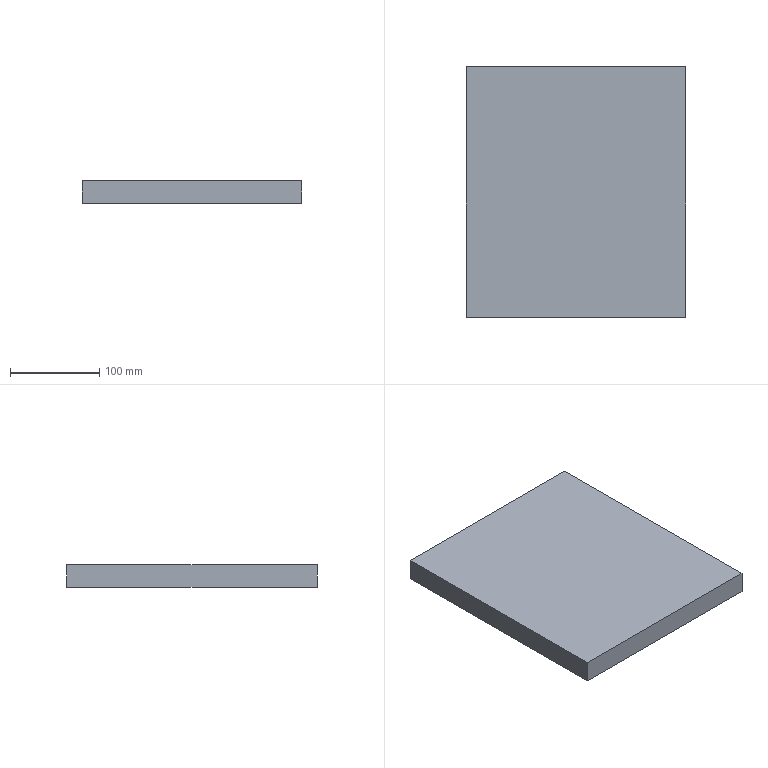Part | SolidWorks | features Extrusion 1 | 1 solid | 6 faces | box 245 x 280 x 25 mm | volume 1715000 mm3 | plane 6
STEP:
#1=CARTESIAN_POINT('',(122.5,-140.,0.));
#2=VERTEX_POINT('',#1);
#3=CARTESIAN_POINT('',(122.5,140.,0.));
#4=VERTEX_POINT('',#3);
#5=CARTESIAN_POINT('',(122.5,140.,0.));
#6=DIRECTION('',(0.,1.,0.));
#7=VECTOR('',#6,1000.);
#8=LINE('',#5,#7);
#9=EDGE_CURVE('',#2,#4,#8,.T.);
#10=ORIENTED_EDGE('',*,*,#9,.T.);
#11=CARTESIAN_POINT('',(122.5,140.,25.));
#12=VERTEX_POINT('',#11);
#13=CARTESIAN_POINT('',(122.5,140.,25.));
#14=DIRECTION('',(0.,0.,-1.));
#15=VECTOR('',#14,1000.);
#16=LINE('',#13,#15);
#17=EDGE_CURVE('',#12,#4,#16,.T.);
#18=ORIENTED_EDGE('',*,*,#17,.F.);
#19=CARTESIAN_POINT('',(122.5,-140.,25.));
#20=VERTEX_POINT('',#19);
#21=CARTESIAN_POINT('',(122.5,140.,25.));
#22=DIRECTION('',(0.,1.,0.));
#23=VECTOR('',#22,1000.);
#24=LINE('',#21,#23);
#25=EDGE_CURVE('',#20,#12,#24,.T.);
#26=ORIENTED_EDGE('',*,*,#25,.F.);
#27=CARTESIAN_POINT('',(122.5,-140.,25.));
#28=DIRECTION('',(0.,0.,-1.));
#29=VECTOR('',#28,1000.);
#30=LINE('',#27,#29);
#31=EDGE_CURVE('',#20,#2,#30,.T.);
#32=ORIENTED_EDGE('',*,*,#31,.T.);
#33=EDGE_LOOP('',(#10,#18,#26,#32));
#34=FACE_OUTER_BOUND('',#33,.T.);
#35=CARTESIAN_POINT('',(122.5,140.,25.));
#36=DIRECTION('',(-1.,0.,0.));
#37=DIRECTION('',(0.,-1.,0.));
#38=AXIS2_PLACEMENT_3D('',#35,#36,#37);
#39=PLANE('',#38);
#40=ADVANCED_FACE('',(#34),#39,.F.);
#41=CARTESIAN_POINT('',(-122.5,140.,0.));
#42=VERTEX_POINT('',#41);
#43=CARTESIAN_POINT('',(-122.5,140.,0.));
#44=DIRECTION('',(-1.,0.,0.));
#45=VECTOR('',#44,1000.);
#46=LINE('',#43,#45);
#47=EDGE_CURVE('',#4,#42,#46,.T.);
#48=ORIENTED_EDGE('',*,*,#47,.T.);
#49=CARTESIAN_POINT('',(-122.5,140.,25.));
#50=VERTEX_POINT('',#49);
#51=CARTESIAN_POINT('',(-122.5,140.,25.));
#52=DIRECTION('',(0.,0.,-1.));
#53=VECTOR('',#52,1000.);
#54=LINE('',#51,#53);
#55=EDGE_CURVE('',#50,#42,#54,.T.);
#56=ORIENTED_EDGE('',*,*,#55,.F.);
#57=CARTESIAN_POINT('',(-122.5,140.,25.));
#58=DIRECTION('',(-1.,0.,0.));
#59=VECTOR('',#58,1000.);
#60=LINE('',#57,#59);
#61=EDGE_CURVE('',#12,#50,#60,.T.);
#62=ORIENTED_EDGE('',*,*,#61,.F.);
#63=ORIENTED_EDGE('',*,*,#17,.T.);
#64=EDGE_LOOP('',(#48,#56,#62,#63));
#65=FACE_OUTER_BOUND('',#64,.T.);
#66=CARTESIAN_POINT('',(-122.5,140.,25.));
#67=DIRECTION('',(0.,-1.,0.));
#68=DIRECTION('',(1.,0.,0.));
#69=AXIS2_PLACEMENT_3D('',#66,#67,#68);
#70=PLANE('',#69);
#71=ADVANCED_FACE('',(#65),#70,.F.);
#72=CARTESIAN_POINT('',(-122.5,-140.,0.));
#73=VERTEX_POINT('',#72);
#74=CARTESIAN_POINT('',(-122.5,140.,0.));
#75=DIRECTION('',(0.,-1.,0.));
#76=VECTOR('',#75,1000.);
#77=LINE('',#74,#76);
#78=EDGE_CURVE('',#42,#73,#77,.T.);
#79=ORIENTED_EDGE('',*,*,#78,.T.);
#80=CARTESIAN_POINT('',(-122.5,-140.,25.));
#81=VERTEX_POINT('',#80);
#82=CARTESIAN_POINT('',(-122.5,-140.,25.));
#83=DIRECTION('',(0.,0.,-1.));
#84=VECTOR('',#83,1000.);
#85=LINE('',#82,#84);
#86=EDGE_CURVE('',#81,#73,#85,.T.);
#87=ORIENTED_EDGE('',*,*,#86,.F.);
#88=CARTESIAN_POINT('',(-122.5,140.,25.));
#89=DIRECTION('',(0.,-1.,0.));
#90=VECTOR('',#89,1000.);
#91=LINE('',#88,#90);
#92=EDGE_CURVE('',#50,#81,#91,.T.);
#93=ORIENTED_EDGE('',*,*,#92,.F.);
#94=ORIENTED_EDGE('',*,*,#55,.T.);
#95=EDGE_LOOP('',(#79,#87,#93,#94));
#96=FACE_OUTER_BOUND('',#95,.T.);
#97=CARTESIAN_POINT('',(-122.5,140.,25.));
#98=DIRECTION('',(1.,0.,0.));
#99=DIRECTION('',(0.,1.,0.));
#100=AXIS2_PLACEMENT_3D('',#97,#98,#99);
#101=PLANE('',#100);
#102=ADVANCED_FACE('',(#96),#101,.F.);
#103=CARTESIAN_POINT('',(-122.5,-140.,0.));
#104=DIRECTION('',(1.,0.,0.));
#105=VECTOR('',#104,1000.);
#106=LINE('',#103,#105);
#107=EDGE_CURVE('',#73,#2,#106,.T.);
#108=ORIENTED_EDGE('',*,*,#107,.T.);
#109=ORIENTED_EDGE('',*,*,#31,.F.);
#110=CARTESIAN_POINT('',(-122.5,-140.,25.));
#111=DIRECTION('',(1.,0.,0.));
#112=VECTOR('',#111,1000.);
#113=LINE('',#110,#112);
#114=EDGE_CURVE('',#81,#20,#113,.T.);
#115=ORIENTED_EDGE('',*,*,#114,.F.);
#116=ORIENTED_EDGE('',*,*,#86,.T.);
#117=EDGE_LOOP('',(#108,#109,#115,#116));
#118=FACE_OUTER_BOUND('',#117,.T.);
#119=CARTESIAN_POINT('',(-122.5,-140.,25.));
#120=DIRECTION('',(0.,1.,0.));
#121=DIRECTION('',(0.,0.,1.));
#122=AXIS2_PLACEMENT_3D('',#119,#120,#121);
#123=PLANE('',#122);
#124=ADVANCED_FACE('',(#118),#123,.F.);
#125=ORIENTED_EDGE('',*,*,#25,.T.);
#126=ORIENTED_EDGE('',*,*,#61,.T.);
#127=ORIENTED_EDGE('',*,*,#92,.T.);
#128=ORIENTED_EDGE('',*,*,#114,.T.);
#129=EDGE_LOOP('',(#125,#126,#127,#128));
#130=FACE_OUTER_BOUND('',#129,.T.);
#131=CARTESIAN_POINT('',(0.,0.,25.));
#132=DIRECTION('',(0.,0.,1.));
#133=DIRECTION('',(1.,0.,0.));
#134=AXIS2_PLACEMENT_3D('',#131,#132,#133);
#135=PLANE('',#134);
#136=ADVANCED_FACE('',(#130),#135,.T.);
#137=ORIENTED_EDGE('',*,*,#9,.F.);
#138=ORIENTED_EDGE('',*,*,#107,.F.);
#139=ORIENTED_EDGE('',*,*,#78,.F.);
#140=ORIENTED_EDGE('',*,*,#47,.F.);
#141=EDGE_LOOP('',(#137,#138,#139,#140));
#142=FACE_OUTER_BOUND('',#141,.T.);
#143=CARTESIAN_POINT('',(0.,0.,0.));
#144=DIRECTION('',(0.,0.,1.));
#145=DIRECTION('',(1.,0.,0.));
#146=AXIS2_PLACEMENT_3D('',#143,#144,#145);
#147=PLANE('',#146);
#148=ADVANCED_FACE('',(#142),#147,.F.);
#149=CLOSED_SHELL('',(#40,#71,#102,#124,#136,#148));
#150=MANIFOLD_SOLID_BREP('',#149);
#151=CARTESIAN_POINT('',(0.,0.,0.));
#152=DIRECTION('',(0.,0.,1.));
#153=DIRECTION('',(1.,0.,0.));
#154=AXIS2_PLACEMENT_3D('',#151,#152,#153);
#155=(LENGTH_UNIT()NAMED_UNIT(*)SI_UNIT(.MILLI.,.METRE.));
#156=UNCERTAINTY_MEASURE_WITH_UNIT(LENGTH_MEASURE(0.00001),#155,'','');
#157=(NAMED_UNIT(*)PLANE_ANGLE_UNIT()SI_UNIT($,.RADIAN.));
#158=(NAMED_UNIT(*)SI_UNIT($,.STERADIAN.)SOLID_ANGLE_UNIT());
#159=(GEOMETRIC_REPRESENTATION_CONTEXT(3)GLOBAL_UNCERTAINTY_ASSIGNED_CONTEXT((#156))GLOBAL_UNIT_ASSIGNED_CONTEXT((#155,#157,#158))REPRESENTATION_CONTEXT('',''));
#160=ADVANCED_BREP_SHAPE_REPRESENTATION('',(#150,#154),#159);